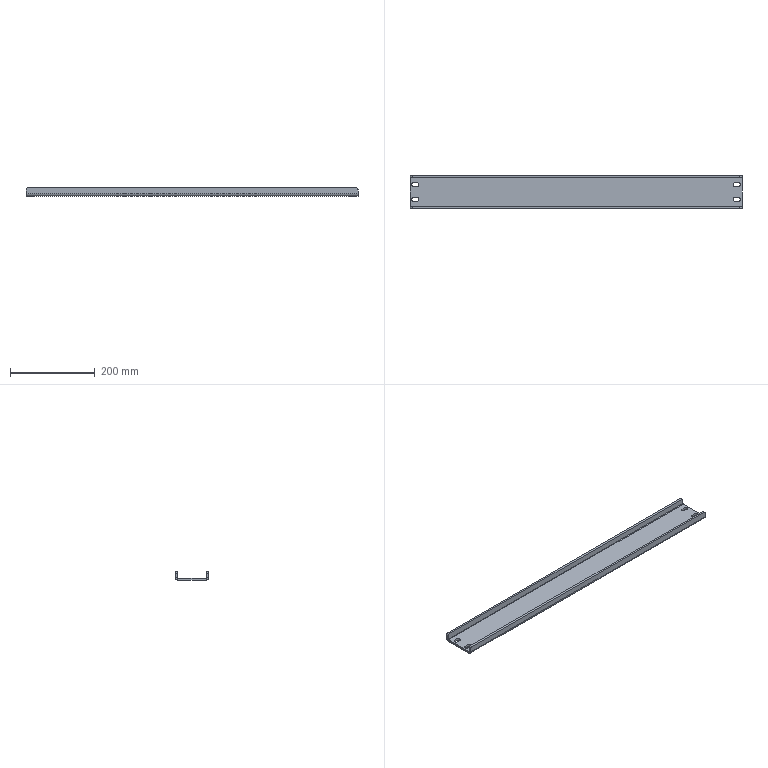Part | SolidWorks | features EdgeFlange 1, Fillet 1, FlatPattern 1, ICE 1, SMBaseFlange 1, SheetMetal 1 | 1 solid | 46 faces | box 785 x 80 x 20 mm | volume 417138 mm3 | plane 26 | cylinder 20 | commonest cylinder face diameters 9 x12 10 x4 2 x2 12 x2
STEP:
#1=CARTESIAN_POINT('',(781.,-22.5,-5.));
#2=VERTEX_POINT('',#1);
#3=CARTESIAN_POINT('',(776.5,-18.,-5.));
#4=VERTEX_POINT('',#3);
#5=CARTESIAN_POINT('',(776.5,-22.5,-5.));
#6=DIRECTION('',(0.,0.,1.));
#7=DIRECTION('',(1.,0.,0.));
#8=AXIS2_PLACEMENT_3D('',#5,#6,#7);
#9=CIRCLE('',#8,4.5);
#10=EDGE_CURVE('',#2,#4,#9,.T.);
#11=ORIENTED_EDGE('',*,*,#10,.F.);
#12=CARTESIAN_POINT('',(781.,-22.5,0.));
#13=VERTEX_POINT('',#12);
#14=CARTESIAN_POINT('',(781.,-22.5,-10.));
#15=DIRECTION('',(0.,0.,1.));
#16=VECTOR('',#15,1000.);
#17=LINE('',#14,#16);
#18=EDGE_CURVE('',#2,#13,#17,.T.);
#19=ORIENTED_EDGE('',*,*,#18,.T.);
#20=CARTESIAN_POINT('',(776.5,-18.,0.));
#21=VERTEX_POINT('',#20);
#22=CARTESIAN_POINT('',(776.5,-22.5,0.));
#23=DIRECTION('',(0.,0.,1.));
#24=DIRECTION('',(-1.,0.,0.));
#25=AXIS2_PLACEMENT_3D('',#22,#23,#24);
#26=CIRCLE('',#25,4.5);
#27=EDGE_CURVE('',#13,#21,#26,.T.);
#28=ORIENTED_EDGE('',*,*,#27,.T.);
#29=CARTESIAN_POINT('',(776.5,-18.,-10.));
#30=DIRECTION('',(0.,0.,1.));
#31=VECTOR('',#30,1000.);
#32=LINE('',#29,#31);
#33=EDGE_CURVE('',#4,#21,#32,.T.);
#34=ORIENTED_EDGE('',*,*,#33,.F.);
#35=EDGE_LOOP('',(#11,#19,#28,#34));
#36=FACE_OUTER_BOUND('',#35,.T.);
#37=CARTESIAN_POINT('',(776.5,-22.5,-10.));
#38=DIRECTION('',(0.,0.,1.));
#39=DIRECTION('',(1.,0.,0.));
#40=AXIS2_PLACEMENT_3D('',#37,#38,#39);
#41=CYLINDRICAL_SURFACE('',#40,4.5);
#42=ADVANCED_FACE('',(#36),#41,.F.);
#43=CARTESIAN_POINT('',(781.,-57.5,-5.));
#44=VERTEX_POINT('',#43);
#45=CARTESIAN_POINT('',(776.5,-53.,-5.));
#46=VERTEX_POINT('',#45);
#47=CARTESIAN_POINT('',(776.5,-57.5,-5.));
#48=DIRECTION('',(0.,0.,1.));
#49=DIRECTION('',(1.,0.,0.));
#50=AXIS2_PLACEMENT_3D('',#47,#48,#49);
#51=CIRCLE('',#50,4.5);
#52=EDGE_CURVE('',#44,#46,#51,.T.);
#53=ORIENTED_EDGE('',*,*,#52,.F.);
#54=CARTESIAN_POINT('',(781.,-57.5,0.));
#55=VERTEX_POINT('',#54);
#56=CARTESIAN_POINT('',(781.,-57.5,-10.));
#57=DIRECTION('',(0.,0.,1.));
#58=VECTOR('',#57,1000.);
#59=LINE('',#56,#58);
#60=EDGE_CURVE('',#44,#55,#59,.T.);
#61=ORIENTED_EDGE('',*,*,#60,.T.);
#62=CARTESIAN_POINT('',(776.5,-53.,0.));
#63=VERTEX_POINT('',#62);
#64=CARTESIAN_POINT('',(776.5,-57.5,0.));
#65=DIRECTION('',(0.,0.,1.));
#66=DIRECTION('',(-1.,0.,0.));
#67=AXIS2_PLACEMENT_3D('',#64,#65,#66);
#68=CIRCLE('',#67,4.5);
#69=EDGE_CURVE('',#55,#63,#68,.T.);
#70=ORIENTED_EDGE('',*,*,#69,.T.);
#71=CARTESIAN_POINT('',(776.5,-53.,-10.));
#72=DIRECTION('',(0.,0.,1.));
#73=VECTOR('',#72,1000.);
#74=LINE('',#71,#73);
#75=EDGE_CURVE('',#46,#63,#74,.T.);
#76=ORIENTED_EDGE('',*,*,#75,.F.);
#77=EDGE_LOOP('',(#53,#61,#70,#76));
#78=FACE_OUTER_BOUND('',#77,.T.);
#79=CARTESIAN_POINT('',(776.5,-57.5,-10.));
#80=DIRECTION('',(0.,0.,1.));
#81=DIRECTION('',(1.,0.,0.));
#82=AXIS2_PLACEMENT_3D('',#79,#80,#81);
#83=CYLINDRICAL_SURFACE('',#82,4.5);
#84=ADVANCED_FACE('',(#78),#83,.F.);
#85=CARTESIAN_POINT('',(21.,-57.5,-5.));
#86=VERTEX_POINT('',#85);
#87=CARTESIAN_POINT('',(16.5,-53.,-5.));
#88=VERTEX_POINT('',#87);
#89=CARTESIAN_POINT('',(16.5,-57.5,-5.));
#90=DIRECTION('',(0.,0.,1.));
#91=DIRECTION('',(1.,0.,0.));
#92=AXIS2_PLACEMENT_3D('',#89,#90,#91);
#93=CIRCLE('',#92,4.5);
#94=EDGE_CURVE('',#86,#88,#93,.T.);
#95=ORIENTED_EDGE('',*,*,#94,.F.);
#96=CARTESIAN_POINT('',(21.,-57.5,0.));
#97=VERTEX_POINT('',#96);
#98=CARTESIAN_POINT('',(21.,-57.5,-10.));
#99=DIRECTION('',(0.,0.,1.));
#100=VECTOR('',#99,1000.);
#101=LINE('',#98,#100);
#102=EDGE_CURVE('',#86,#97,#101,.T.);
#103=ORIENTED_EDGE('',*,*,#102,.T.);
#104=CARTESIAN_POINT('',(16.5,-53.,0.));
#105=VERTEX_POINT('',#104);
#106=CARTESIAN_POINT('',(16.5,-57.5,0.));
#107=DIRECTION('',(0.,0.,1.));
#108=DIRECTION('',(1.,0.,0.));
#109=AXIS2_PLACEMENT_3D('',#106,#107,#108);
#110=CIRCLE('',#109,4.5);
#111=EDGE_CURVE('',#97,#105,#110,.T.);
#112=ORIENTED_EDGE('',*,*,#111,.T.);
#113=CARTESIAN_POINT('',(16.5,-53.,-10.));
#114=DIRECTION('',(0.,0.,1.));
#115=VECTOR('',#114,1000.);
#116=LINE('',#113,#115);
#117=EDGE_CURVE('',#88,#105,#116,.T.);
#118=ORIENTED_EDGE('',*,*,#117,.F.);
#119=EDGE_LOOP('',(#95,#103,#112,#118));
#120=FACE_OUTER_BOUND('',#119,.T.);
#121=CARTESIAN_POINT('',(16.5,-57.5,-10.));
#122=DIRECTION('',(0.,0.,1.));
#123=DIRECTION('',(1.,0.,0.));
#124=AXIS2_PLACEMENT_3D('',#121,#122,#123);
#125=CYLINDRICAL_SURFACE('',#124,4.5);
#126=ADVANCED_FACE('',(#120),#125,.F.);
#127=CARTESIAN_POINT('',(21.,-22.5,-5.));
#128=VERTEX_POINT('',#127);
#129=CARTESIAN_POINT('',(16.5,-18.,-5.));
#130=VERTEX_POINT('',#129);
#131=CARTESIAN_POINT('',(16.5,-22.5,-5.));
#132=DIRECTION('',(0.,0.,1.));
#133=DIRECTION('',(1.,0.,0.));
#134=AXIS2_PLACEMENT_3D('',#131,#132,#133);
#135=CIRCLE('',#134,4.5);
#136=EDGE_CURVE('',#128,#130,#135,.T.);
#137=ORIENTED_EDGE('',*,*,#136,.F.);
#138=CARTESIAN_POINT('',(21.,-22.5,0.));
#139=VERTEX_POINT('',#138);
#140=CARTESIAN_POINT('',(21.,-22.5,-10.));
#141=DIRECTION('',(0.,0.,1.));
#142=VECTOR('',#141,1000.);
#143=LINE('',#140,#142);
#144=EDGE_CURVE('',#128,#139,#143,.T.);
#145=ORIENTED_EDGE('',*,*,#144,.T.);
#146=CARTESIAN_POINT('',(16.5,-18.,0.));
#147=VERTEX_POINT('',#146);
#148=CARTESIAN_POINT('',(16.5,-22.5,0.));
#149=DIRECTION('',(0.,0.,1.));
#150=DIRECTION('',(1.,0.,0.));
#151=AXIS2_PLACEMENT_3D('',#148,#149,#150);
#152=CIRCLE('',#151,4.5);
#153=EDGE_CURVE('',#139,#147,#152,.T.);
#154=ORIENTED_EDGE('',*,*,#153,.T.);
#155=CARTESIAN_POINT('',(16.5,-18.,-10.));
#156=DIRECTION('',(0.,0.,1.));
#157=VECTOR('',#156,1000.);
#158=LINE('',#155,#157);
#159=EDGE_CURVE('',#130,#147,#158,.T.);
#160=ORIENTED_EDGE('',*,*,#159,.F.);
#161=EDGE_LOOP('',(#137,#145,#154,#160));
#162=FACE_OUTER_BOUND('',#161,.T.);
#163=CARTESIAN_POINT('',(16.5,-22.5,-10.));
#164=DIRECTION('',(0.,0.,1.));
#165=DIRECTION('',(1.,0.,0.));
#166=AXIS2_PLACEMENT_3D('',#163,#164,#165);
#167=CYLINDRICAL_SURFACE('',#166,4.5);
#168=ADVANCED_FACE('',(#162),#167,.F.);
#169=CARTESIAN_POINT('',(768.5,-27.,-5.));
#170=VERTEX_POINT('',#169);
#171=CARTESIAN_POINT('',(776.5,-27.,-5.));
#172=VERTEX_POINT('',#171);
#173=CARTESIAN_POINT('',(0.,-27.,-5.));
#174=DIRECTION('',(1.,0.,0.));
#175=VECTOR('',#174,1000.);
#176=LINE('',#173,#175);
#177=EDGE_CURVE('',#170,#172,#176,.T.);
#178=ORIENTED_EDGE('',*,*,#177,.T.);
#179=CARTESIAN_POINT('',(776.5,-22.5,-5.));
#180=DIRECTION('',(0.,0.,1.));
#181=DIRECTION('',(1.,0.,0.));
#182=AXIS2_PLACEMENT_3D('',#179,#180,#181);
#183=CIRCLE('',#182,4.5);
#184=EDGE_CURVE('',#172,#2,#183,.T.);
#185=ORIENTED_EDGE('',*,*,#184,.T.);
#186=ORIENTED_EDGE('',*,*,#10,.T.);
#187=CARTESIAN_POINT('',(768.5,-18.,-5.));
#188=VERTEX_POINT('',#187);
#189=CARTESIAN_POINT('',(0.,-18.,-5.));
#190=DIRECTION('',(-1.,0.,0.));
#191=VECTOR('',#190,1000.);
#192=LINE('',#189,#191);
#193=EDGE_CURVE('',#4,#188,#192,.T.);
#194=ORIENTED_EDGE('',*,*,#193,.T.);
#195=CARTESIAN_POINT('',(768.5,-22.5,-5.));
#196=DIRECTION('',(0.,0.,1.));
#197=DIRECTION('',(1.,0.,0.));
#198=AXIS2_PLACEMENT_3D('',#195,#196,#197);
#199=CIRCLE('',#198,4.5);
#200=EDGE_CURVE('',#188,#170,#199,.T.);
#201=ORIENTED_EDGE('',*,*,#200,.T.);
#202=EDGE_LOOP('',(#178,#185,#186,#194,#201));
#203=FACE_BOUND('',#202,.T.);
#204=CARTESIAN_POINT('',(768.5,-62.,-5.));
#205=VERTEX_POINT('',#204);
#206=CARTESIAN_POINT('',(776.5,-62.,-5.));
#207=VERTEX_POINT('',#206);
#208=CARTESIAN_POINT('',(0.,-62.,-5.));
#209=DIRECTION('',(1.,0.,0.));
#210=VECTOR('',#209,1000.);
#211=LINE('',#208,#210);
#212=EDGE_CURVE('',#205,#207,#211,.T.);
#213=ORIENTED_EDGE('',*,*,#212,.T.);
#214=CARTESIAN_POINT('',(776.5,-57.5,-5.));
#215=DIRECTION('',(0.,0.,1.));
#216=DIRECTION('',(1.,0.,0.));
#217=AXIS2_PLACEMENT_3D('',#214,#215,#216);
#218=CIRCLE('',#217,4.5);
#219=EDGE_CURVE('',#207,#44,#218,.T.);
#220=ORIENTED_EDGE('',*,*,#219,.T.);
#221=ORIENTED_EDGE('',*,*,#52,.T.);
#222=CARTESIAN_POINT('',(768.5,-53.,-5.));
#223=VERTEX_POINT('',#222);
#224=CARTESIAN_POINT('',(0.,-53.,-5.));
#225=DIRECTION('',(-1.,0.,0.));
#226=VECTOR('',#225,1000.);
#227=LINE('',#224,#226);
#228=EDGE_CURVE('',#46,#223,#227,.T.);
#229=ORIENTED_EDGE('',*,*,#228,.T.);
#230=CARTESIAN_POINT('',(768.5,-57.5,-5.));
#231=DIRECTION('',(0.,0.,1.));
#232=DIRECTION('',(1.,0.,0.));
#233=AXIS2_PLACEMENT_3D('',#230,#231,#232);
#234=CIRCLE('',#233,4.5);
#235=EDGE_CURVE('',#223,#205,#234,.T.);
#236=ORIENTED_EDGE('',*,*,#235,.T.);
#237=EDGE_LOOP('',(#213,#220,#221,#229,#236));
#238=FACE_BOUND('',#237,.T.);
#239=CARTESIAN_POINT('',(8.5,-53.,-5.));
#240=VERTEX_POINT('',#239);
#241=CARTESIAN_POINT('',(0.,-53.,-5.));
#242=DIRECTION('',(-1.,0.,0.));
#243=VECTOR('',#242,1000.);
#244=LINE('',#241,#243);
#245=EDGE_CURVE('',#88,#240,#244,.T.);
#246=ORIENTED_EDGE('',*,*,#245,.T.);
#247=CARTESIAN_POINT('',(8.5,-62.,-5.));
#248=VERTEX_POINT('',#247);
#249=CARTESIAN_POINT('',(8.5,-57.5,-5.));
#250=DIRECTION('',(0.,0.,1.));
#251=DIRECTION('',(1.,0.,0.));
#252=AXIS2_PLACEMENT_3D('',#249,#250,#251);
#253=CIRCLE('',#252,4.5);
#254=EDGE_CURVE('',#240,#248,#253,.T.);
#255=ORIENTED_EDGE('',*,*,#254,.T.);
#256=CARTESIAN_POINT('',(16.5,-62.,-5.));
#257=VERTEX_POINT('',#256);
#258=CARTESIAN_POINT('',(0.,-62.,-5.));
#259=DIRECTION('',(1.,0.,0.));
#260=VECTOR('',#259,1000.);
#261=LINE('',#258,#260);
#262=EDGE_CURVE('',#248,#257,#261,.T.);
#263=ORIENTED_EDGE('',*,*,#262,.T.);
#264=CARTESIAN_POINT('',(16.5,-57.5,-5.));
#265=DIRECTION('',(0.,0.,1.));
#266=DIRECTION('',(1.,0.,0.));
#267=AXIS2_PLACEMENT_3D('',#264,#265,#266);
#268=CIRCLE('',#267,4.5);
#269=EDGE_CURVE('',#257,#86,#268,.T.);
#270=ORIENTED_EDGE('',*,*,#269,.T.);
#271=ORIENTED_EDGE('',*,*,#94,.T.);
#272=EDGE_LOOP('',(#246,#255,#263,#270,#271));
#273=FACE_BOUND('',#272,.T.);
#274=CARTESIAN_POINT('',(8.5,-18.,-5.));
#275=VERTEX_POINT('',#274);
#276=CARTESIAN_POINT('',(0.,-18.,-5.));
#277=DIRECTION('',(-1.,0.,0.));
#278=VECTOR('',#277,1000.);
#279=LINE('',#276,#278);
#280=EDGE_CURVE('',#130,#275,#279,.T.);
#281=ORIENTED_EDGE('',*,*,#280,.T.);
#282=CARTESIAN_POINT('',(8.5,-27.,-5.));
#283=VERTEX_POINT('',#282);
#284=CARTESIAN_POINT('',(8.5,-22.5,-5.));
#285=DIRECTION('',(0.,0.,1.));
#286=DIRECTION('',(1.,0.,0.));
#287=AXIS2_PLACEMENT_3D('',#284,#285,#286);
#288=CIRCLE('',#287,4.5);
#289=EDGE_CURVE('',#275,#283,#288,.T.);
#290=ORIENTED_EDGE('',*,*,#289,.T.);
#291=CARTESIAN_POINT('',(16.5,-27.,-5.));
#292=VERTEX_POINT('',#291);
#293=CARTESIAN_POINT('',(0.,-27.,-5.));
#294=DIRECTION('',(1.,0.,0.));
#295=VECTOR('',#294,1000.);
#296=LINE('',#293,#295);
#297=EDGE_CURVE('',#283,#292,#296,.T.);
#298=ORIENTED_EDGE('',*,*,#297,.T.);
#299=CARTESIAN_POINT('',(16.5,-22.5,-5.));
#300=DIRECTION('',(0.,0.,1.));
#301=DIRECTION('',(1.,0.,0.));
#302=AXIS2_PLACEMENT_3D('',#299,#300,#301);
#303=CIRCLE('',#302,4.5);
#304=EDGE_CURVE('',#292,#128,#303,.T.);
#305=ORIENTED_EDGE('',*,*,#304,.T.);
#306=ORIENTED_EDGE('',*,*,#136,.T.);
#307=EDGE_LOOP('',(#281,#290,#298,#305,#306));
#308=FACE_BOUND('',#307,.T.);
#309=CARTESIAN_POINT('',(785.,-74.,-5.));
#310=VERTEX_POINT('',#309);
#311=CARTESIAN_POINT('',(0.,-74.,-5.));
#312=VERTEX_POINT('',#311);
#313=CARTESIAN_POINT('',(785.,-74.,-5.));
#314=DIRECTION('',(-1.,0.,0.));
#315=VECTOR('',#314,1000.);
#316=LINE('',#313,#315);
#317=EDGE_CURVE('',#310,#312,#316,.T.);
#318=ORIENTED_EDGE('',*,*,#317,.T.);
#319=CARTESIAN_POINT('',(0.,-6.,-5.));
#320=VERTEX_POINT('',#319);
#321=CARTESIAN_POINT('',(0.,0.,-5.));
#322=DIRECTION('',(0.,-1.,0.));
#323=VECTOR('',#322,1000.);
#324=LINE('',#321,#323);
#325=EDGE_CURVE('',#320,#312,#324,.T.);
#326=ORIENTED_EDGE('',*,*,#325,.F.);
#327=CARTESIAN_POINT('',(785.,-6.,-5.));
#328=VERTEX_POINT('',#327);
#329=CARTESIAN_POINT('',(0.,-6.,-5.));
#330=DIRECTION('',(1.,0.,0.));
#331=VECTOR('',#330,1000.);
#332=LINE('',#329,#331);
#333=EDGE_CURVE('',#320,#328,#332,.T.);
#334=ORIENTED_EDGE('',*,*,#333,.T.);
#335=CARTESIAN_POINT('',(785.,0.,-5.));
#336=DIRECTION('',(0.,1.,0.));
#337=VECTOR('',#336,1000.);
#338=LINE('',#335,#337);
#339=EDGE_CURVE('',#310,#328,#338,.T.);
#340=ORIENTED_EDGE('',*,*,#339,.F.);
#341=EDGE_LOOP('',(#318,#326,#334,#340));
#342=FACE_OUTER_BOUND('',#341,.T.);
#343=CARTESIAN_POINT('',(0.,0.,-5.));
#344=DIRECTION('',(0.,0.,1.));
#345=DIRECTION('',(1.,0.,0.));
#346=AXIS2_PLACEMENT_3D('',#343,#344,#345);
#347=PLANE('',#346);
#348=ADVANCED_FACE('',(#203,#238,#273,#308,#342),#347,.F.);
#349=CARTESIAN_POINT('',(776.5,-27.,0.));
#350=VERTEX_POINT('',#349);
#351=CARTESIAN_POINT('',(776.5,-22.5,0.));
#352=DIRECTION('',(0.,0.,1.));
#353=DIRECTION('',(-1.,0.,0.));
#354=AXIS2_PLACEMENT_3D('',#351,#352,#353);
#355=CIRCLE('',#354,4.5);
#356=EDGE_CURVE('',#350,#13,#355,.T.);
#357=ORIENTED_EDGE('',*,*,#356,.F.);
#358=CARTESIAN_POINT('',(768.5,-27.,0.));
#359=VERTEX_POINT('',#358);
#360=CARTESIAN_POINT('',(776.5,-27.,0.));
#361=DIRECTION('',(1.,0.,0.));
#362=VECTOR('',#361,1000.);
#363=LINE('',#360,#362);
#364=EDGE_CURVE('',#359,#350,#363,.T.);
#365=ORIENTED_EDGE('',*,*,#364,.F.);
#366=CARTESIAN_POINT('',(768.5,-18.,0.));
#367=VERTEX_POINT('',#366);
#368=CARTESIAN_POINT('',(768.5,-22.5,0.));
#369=DIRECTION('',(0.,0.,1.));
#370=DIRECTION('',(-1.,0.,0.));
#371=AXIS2_PLACEMENT_3D('',#368,#369,#370);
#372=CIRCLE('',#371,4.5);
#373=EDGE_CURVE('',#367,#359,#372,.T.);
#374=ORIENTED_EDGE('',*,*,#373,.F.);
#375=CARTESIAN_POINT('',(776.5,-18.,0.));
#376=DIRECTION('',(-1.,0.,0.));
#377=VECTOR('',#376,1000.);
#378=LINE('',#375,#377);
#379=EDGE_CURVE('',#21,#367,#378,.T.);
#380=ORIENTED_EDGE('',*,*,#379,.F.);
#381=ORIENTED_EDGE('',*,*,#27,.F.);
#382=EDGE_LOOP('',(#357,#365,#374,#380,#381));
#383=FACE_BOUND('',#382,.T.);
#384=CARTESIAN_POINT('',(776.5,-62.,0.));
#385=VERTEX_POINT('',#384);
#386=CARTESIAN_POINT('',(776.5,-57.5,0.));
#387=DIRECTION('',(0.,0.,1.));
#388=DIRECTION('',(-1.,0.,0.));
#389=AXIS2_PLACEMENT_3D('',#386,#387,#388);
#390=CIRCLE('',#389,4.5);
#391=EDGE_CURVE('',#385,#55,#390,.T.);
#392=ORIENTED_EDGE('',*,*,#391,.F.);
#393=CARTESIAN_POINT('',(768.5,-62.,0.));
#394=VERTEX_POINT('',#393);
#395=CARTESIAN_POINT('',(776.5,-62.,0.));
#396=DIRECTION('',(1.,0.,0.));
#397=VECTOR('',#396,1000.);
#398=LINE('',#395,#397);
#399=EDGE_CURVE('',#394,#385,#398,.T.);
#400=ORIENTED_EDGE('',*,*,#399,.F.);
#401=CARTESIAN_POINT('',(768.5,-53.,0.));
#402=VERTEX_POINT('',#401);
#403=CARTESIAN_POINT('',(768.5,-57.5,0.));
#404=DIRECTION('',(0.,0.,1.));
#405=DIRECTION('',(-1.,0.,0.));
#406=AXIS2_PLACEMENT_3D('',#403,#404,#405);
#407=CIRCLE('',#406,4.5);
#408=EDGE_CURVE('',#402,#394,#407,.T.);
#409=ORIENTED_EDGE('',*,*,#408,.F.);
#410=CARTESIAN_POINT('',(776.5,-53.,0.));
#411=DIRECTION('',(-1.,0.,0.));
#412=VECTOR('',#411,1000.);
#413=LINE('',#410,#412);
#414=EDGE_CURVE('',#63,#402,#413,.T.);
#415=ORIENTED_EDGE('',*,*,#414,.F.);
#416=ORIENTED_EDGE('',*,*,#69,.F.);
#417=EDGE_LOOP('',(#392,#400,#409,#415,#416));
#418=FACE_BOUND('',#417,.T.);
#419=CARTESIAN_POINT('',(8.5,-53.,0.));
#420=VERTEX_POINT('',#419);
#421=CARTESIAN_POINT('',(8.5,-62.,0.));
#422=VERTEX_POINT('',#421);
#423=CARTESIAN_POINT('',(8.5,-57.5,0.));
#424=DIRECTION('',(0.,0.,1.));
#425=DIRECTION('',(1.,0.,0.));
#426=AXIS2_PLACEMENT_3D('',#423,#424,#425);
#427=CIRCLE('',#426,4.5);
#428=EDGE_CURVE('',#420,#422,#427,.T.);
#429=ORIENTED_EDGE('',*,*,#428,.F.);
#430=CARTESIAN_POINT('',(8.5,-53.,0.));
#431=DIRECTION('',(-1.,0.,0.));
#432=VECTOR('',#431,1000.);
#433=LINE('',#430,#432);
#434=EDGE_CURVE('',#105,#420,#433,.T.);
#435=ORIENTED_EDGE('',*,*,#434,.F.);
#436=ORIENTED_EDGE('',*,*,#111,.F.);
#437=CARTESIAN_POINT('',(16.5,-62.,0.));
#438=VERTEX_POINT('',#437);
#439=CARTESIAN_POINT('',(16.5,-57.5,0.));
#440=DIRECTION('',(0.,0.,1.));
#441=DIRECTION('',(1.,0.,0.));
#442=AXIS2_PLACEMENT_3D('',#439,#440,#441);
#443=CIRCLE('',#442,4.5);
#444=EDGE_CURVE('',#438,#97,#443,.T.);
#445=ORIENTED_EDGE('',*,*,#444,.F.);
#446=CARTESIAN_POINT('',(8.5,-62.,0.));
#447=DIRECTION('',(1.,0.,0.));
#448=VECTOR('',#447,1000.);
#449=LINE('',#446,#448);
#450=EDGE_CURVE('',#422,#438,#449,.T.);
#451=ORIENTED_EDGE('',*,*,#450,.F.);
#452=EDGE_LOOP('',(#429,#435,#436,#445,#451));
#453=FACE_BOUND('',#452,.T.);
#454=CARTESIAN_POINT('',(8.5,-18.,0.));
#455=VERTEX_POINT('',#454);
#456=CARTESIAN_POINT('',(8.5,-27.,0.));
#457=VERTEX_POINT('',#456);
#458=CARTESIAN_POINT('',(8.5,-22.5,0.));
#459=DIRECTION('',(0.,0.,1.));
#460=DIRECTION('',(1.,0.,0.));
#461=AXIS2_PLACEMENT_3D('',#458,#459,#460);
#462=CIRCLE('',#461,4.5);
#463=EDGE_CURVE('',#455,#457,#462,.T.);
#464=ORIENTED_EDGE('',*,*,#463,.F.);
#465=CARTESIAN_POINT('',(8.5,-18.,0.));
#466=DIRECTION('',(-1.,0.,0.));
#467=VECTOR('',#466,1000.);
#468=LINE('',#465,#467);
#469=EDGE_CURVE('',#147,#455,#468,.T.);
#470=ORIENTED_EDGE('',*,*,#469,.F.);
#471=ORIENTED_EDGE('',*,*,#153,.F.);
#472=CARTESIAN_POINT('',(16.5,-27.,0.));
#473=VERTEX_POINT('',#472);
#474=CARTESIAN_POINT('',(16.5,-22.5,0.));
#475=DIRECTION('',(0.,0.,1.));
#476=DIRECTION('',(1.,0.,0.));
#477=AXIS2_PLACEMENT_3D('',#474,#475,#476);
#478=CIRCLE('',#477,4.5);
#479=EDGE_CURVE('',#473,#139,#478,.T.);
#480=ORIENTED_EDGE('',*,*,#479,.F.);
#481=CARTESIAN_POINT('',(8.5,-27.,0.));
#482=DIRECTION('',(1.,0.,0.));
#483=VECTOR('',#482,1000.);
#484=LINE('',#481,#483);
#485=EDGE_CURVE('',#457,#473,#484,.T.);
#486=ORIENTED_EDGE('',*,*,#485,.F.);
#487=EDGE_LOOP('',(#464,#470,#471,#480,#486));
#488=FACE_BOUND('',#487,.T.);
#489=CARTESIAN_POINT('',(0.,-6.,0.));
#490=VERTEX_POINT('',#489);
#491=CARTESIAN_POINT('',(0.,-74.,0.));
#492=VERTEX_POINT('',#491);
#493=CARTESIAN_POINT('',(0.,0.,0.));
#494=DIRECTION('',(0.,-1.,0.));
#495=VECTOR('',#494,1000.);
#496=LINE('',#493,#495);
#497=EDGE_CURVE('',#490,#492,#496,.T.);
#498=ORIENTED_EDGE('',*,*,#497,.T.);
#499=CARTESIAN_POINT('',(785.,-74.,0.));
#500=VERTEX_POINT('',#499);
#501=CARTESIAN_POINT('',(785.,-74.,0.));
#502=DIRECTION('',(-1.,0.,0.));
#503=VECTOR('',#502,1000.);
#504=LINE('',#501,#503);
#505=EDGE_CURVE('',#500,#492,#504,.T.);
#506=ORIENTED_EDGE('',*,*,#505,.F.);
#507=CARTESIAN_POINT('',(785.,-6.,0.));
#508=VERTEX_POINT('',#507);
#509=CARTESIAN_POINT('',(785.,0.,0.));
#510=DIRECTION('',(0.,1.,0.));
#511=VECTOR('',#510,1000.);
#512=LINE('',#509,#511);
#513=EDGE_CURVE('',#500,#508,#512,.T.);
#514=ORIENTED_EDGE('',*,*,#513,.T.);
#515=CARTESIAN_POINT('',(0.,-6.,0.));
#516=DIRECTION('',(1.,0.,0.));
#517=VECTOR('',#516,1000.);
#518=LINE('',#515,#517);
#519=EDGE_CURVE('',#490,#508,#518,.T.);
#520=ORIENTED_EDGE('',*,*,#519,.F.);
#521=EDGE_LOOP('',(#498,#506,#514,#520));
#522=FACE_OUTER_BOUND('',#521,.T.);
#523=CARTESIAN_POINT('',(0.,0.,0.));
#524=DIRECTION('',(0.,0.,1.));
#525=DIRECTION('',(1.,0.,0.));
#526=AXIS2_PLACEMENT_3D('',#523,#524,#525);
#527=PLANE('',#526);
#528=ADVANCED_FACE('',(#383,#418,#453,#488,#522),#527,.T.);
#529=ORIENTED_EDGE('',*,*,#513,.F.);
#530=CARTESIAN_POINT('',(785.,-74.,0.));
#531=DIRECTION('',(0.,0.,-1.));
#532=VECTOR('',#531,1000.);
#533=LINE('',#530,#532);
#534=EDGE_CURVE('',#500,#310,#533,.T.);
#535=ORIENTED_EDGE('',*,*,#534,.T.);
#536=ORIENTED_EDGE('',*,*,#339,.T.);
#537=CARTESIAN_POINT('',(785.,-6.,0.));
#538=DIRECTION('',(0.,0.,-1.));
#539=VECTOR('',#538,1000.);
#540=LINE('',#537,#539);
#541=EDGE_CURVE('',#508,#328,#540,.T.);
#542=ORIENTED_EDGE('',*,*,#541,.F.);
#543=EDGE_LOOP('',(#529,#535,#536,#542));
#544=FACE_OUTER_BOUND('',#543,.T.);
#545=CARTESIAN_POINT('',(785.,0.,-5.));
#546=DIRECTION('',(1.,0.,0.));
#547=DIRECTION('',(0.,0.,-1.));
#548=AXIS2_PLACEMENT_3D('',#545,#546,#547);
#549=PLANE('',#548);
#550=ADVANCED_FACE('',(#544),#549,.T.);
#551=CARTESIAN_POINT('',(0.,-74.,0.));
#552=DIRECTION('',(0.,0.,-1.));
#553=VECTOR('',#552,1000.);
#554=LINE('',#551,#553);
#555=EDGE_CURVE('',#492,#312,#554,.T.);
#556=ORIENTED_EDGE('',*,*,#555,.F.);
#557=ORIENTED_EDGE('',*,*,#497,.F.);
#558=CARTESIAN_POINT('',(0.,-6.,0.));
#559=DIRECTION('',(0.,0.,-1.));
#560=VECTOR('',#559,1000.);
#561=LINE('',#558,#560);
#562=EDGE_CURVE('',#490,#320,#561,.T.);
#563=ORIENTED_EDGE('',*,*,#562,.T.);
#564=ORIENTED_EDGE('',*,*,#325,.T.);
#565=EDGE_LOOP('',(#556,#557,#563,#564));
#566=FACE_OUTER_BOUND('',#565,.T.);
#567=CARTESIAN_POINT('',(0.,0.,-5.));
#568=DIRECTION('',(-1.,0.,0.));
#569=DIRECTION('',(0.,-1.,0.));
#570=AXIS2_PLACEMENT_3D('',#567,#568,#569);
#571=PLANE('',#570);
#572=ADVANCED_FACE('',(#566),#571,.T.);
#573=CARTESIAN_POINT('',(785.,-5.,1.));
#574=VERTEX_POINT('',#573);
#575=CARTESIAN_POINT('',(785.,0.,1.));
#576=VERTEX_POINT('',#575);
#577=CARTESIAN_POINT('',(785.,0.,1.));
#578=DIRECTION('',(0.,1.,0.));
#579=VECTOR('',#578,1000.);
#580=LINE('',#577,#579);
#581=EDGE_CURVE('',#574,#576,#580,.T.);
#582=ORIENTED_EDGE('',*,*,#581,.F.);
#583=CARTESIAN_POINT('',(785.,-6.,1.));
#584=DIRECTION('',(1.,0.,0.));
#585=DIRECTION('',(0.,0.,1.));
#586=AXIS2_PLACEMENT_3D('',#583,#584,#585);
#587=CIRCLE('',#586,1.);
#588=EDGE_CURVE('',#508,#574,#587,.T.);
#589=ORIENTED_EDGE('',*,*,#588,.F.);
#590=ORIENTED_EDGE('',*,*,#541,.T.);
#591=CARTESIAN_POINT('',(785.,-6.,1.));
#592=DIRECTION('',(1.,0.,0.));
#593=DIRECTION('',(0.,0.,1.));
#594=AXIS2_PLACEMENT_3D('',#591,#592,#593);
#595=CIRCLE('',#594,6.);
#596=EDGE_CURVE('',#328,#576,#595,.T.);
#597=ORIENTED_EDGE('',*,*,#596,.T.);
#598=EDGE_LOOP('',(#582,#589,#590,#597));
#599=FACE_OUTER_BOUND('',#598,.T.);
#600=CARTESIAN_POINT('',(785.,-6.,1.));
#601=DIRECTION('',(1.,0.,0.));
#602=DIRECTION('',(0.,0.,-1.));
#603=AXIS2_PLACEMENT_3D('',#600,#601,#602);
#604=PLANE('',#603);
#605=ADVANCED_FACE('',(#599),#604,.T.);
#606=CARTESIAN_POINT('',(0.,-5.,1.));
#607=VERTEX_POINT('',#606);
#608=CARTESIAN_POINT('',(0.,-6.,1.));
#609=DIRECTION('',(-1.,0.,0.));
#610=DIRECTION('',(0.,0.,1.));
#611=AXIS2_PLACEMENT_3D('',#608,#609,#610);
#612=CIRCLE('',#611,1.);
#613=EDGE_CURVE('',#607,#490,#612,.T.);
#614=ORIENTED_EDGE('',*,*,#613,.F.);
#615=CARTESIAN_POINT('',(0.,0.,1.));
#616=VERTEX_POINT('',#615);
#617=CARTESIAN_POINT('',(0.,-5.,1.));
#618=DIRECTION('',(0.,1.,0.));
#619=VECTOR('',#618,1000.);
#620=LINE('',#617,#619);
#621=EDGE_CURVE('',#607,#616,#620,.T.);
#622=ORIENTED_EDGE('',*,*,#621,.T.);
#623=CARTESIAN_POINT('',(0.,-6.,1.));
#624=DIRECTION('',(-1.,0.,0.));
#625=DIRECTION('',(0.,0.,1.));
#626=AXIS2_PLACEMENT_3D('',#623,#624,#625);
#627=CIRCLE('',#626,6.);
#628=EDGE_CURVE('',#616,#320,#627,.T.);
#629=ORIENTED_EDGE('',*,*,#628,.T.);
#630=ORIENTED_EDGE('',*,*,#562,.F.);
#631=EDGE_LOOP('',(#614,#622,#629,#630));
#632=FACE_OUTER_BOUND('',#631,.T.);
#633=CARTESIAN_POINT('',(0.,-6.,1.));
#634=DIRECTION('',(1.,0.,0.));
#635=DIRECTION('',(0.,0.,-1.));
#636=AXIS2_PLACEMENT_3D('',#633,#634,#635);
#637=PLANE('',#636);
#638=ADVANCED_FACE('',(#632),#637,.F.);
#639=ORIENTED_EDGE('',*,*,#333,.F.);
#640=ORIENTED_EDGE('',*,*,#628,.F.);
#641=CARTESIAN_POINT('',(785.,0.,1.));
#642=DIRECTION('',(1.,0.,0.));
#643=VECTOR('',#642,1000.);
#644=LINE('',#641,#643);
#645=EDGE_CURVE('',#616,#576,#644,.T.);
#646=ORIENTED_EDGE('',*,*,#645,.T.);
#647=ORIENTED_EDGE('',*,*,#596,.F.);
#648=EDGE_LOOP('',(#639,#640,#646,#647));
#649=FACE_OUTER_BOUND('',#648,.T.);
#650=CARTESIAN_POINT('',(0.,-6.,1.));
#651=DIRECTION('',(-1.,0.,0.));
#652=DIRECTION('',(0.,1.,0.));
#653=AXIS2_PLACEMENT_3D('',#650,#651,#652);
#654=CYLINDRICAL_SURFACE('',#653,6.);
#655=ADVANCED_FACE('',(#649),#654,.T.);
#656=ORIENTED_EDGE('',*,*,#519,.T.);
#657=ORIENTED_EDGE('',*,*,#588,.T.);
#658=CARTESIAN_POINT('',(785.,-5.,1.));
#659=DIRECTION('',(-1.,0.,0.));
#660=VECTOR('',#659,1000.);
#661=LINE('',#658,#660);
#662=EDGE_CURVE('',#574,#607,#661,.T.);
#663=ORIENTED_EDGE('',*,*,#662,.T.);
#664=ORIENTED_EDGE('',*,*,#613,.T.);
#665=EDGE_LOOP('',(#656,#657,#663,#664));
#666=FACE_OUTER_BOUND('',#665,.T.);
#667=CARTESIAN_POINT('',(0.,-6.,1.));
#668=DIRECTION('',(-1.,0.,0.));
#669=DIRECTION('',(0.,1.,0.));
#670=AXIS2_PLACEMENT_3D('',#667,#668,#669);
#671=CYLINDRICAL_SURFACE('',#670,1.);
#672=ADVANCED_FACE('',(#666),#671,.F.);
#673=CARTESIAN_POINT('',(785.,0.,10.));
#674=VERTEX_POINT('',#673);
#675=CARTESIAN_POINT('',(785.,0.,0.));
#676=DIRECTION('',(0.,0.,-1.));
#677=VECTOR('',#676,1000.);
#678=LINE('',#675,#677);
#679=EDGE_CURVE('',#674,#576,#678,.T.);
#680=ORIENTED_EDGE('',*,*,#679,.F.);
#681=CARTESIAN_POINT('',(785.,-5.,10.));
#682=VERTEX_POINT('',#681);
#683=CARTESIAN_POINT('',(785.,0.,10.));
#684=DIRECTION('',(0.,-1.,0.));
#685=VECTOR('',#684,1000.);
#686=LINE('',#683,#685);
#687=EDGE_CURVE('',#674,#682,#686,.T.);
#688=ORIENTED_EDGE('',*,*,#687,.T.);
#689=CARTESIAN_POINT('',(785.,-5.,0.));
#690=DIRECTION('',(0.,0.,-1.));
#691=VECTOR('',#690,1000.);
#692=LINE('',#689,#691);
#693=EDGE_CURVE('',#682,#574,#692,.T.);
#694=ORIENTED_EDGE('',*,*,#693,.T.);
#695=ORIENTED_EDGE('',*,*,#581,.T.);
#696=EDGE_LOOP('',(#680,#688,#694,#695));
#697=FACE_OUTER_BOUND('',#696,.T.);
#698=CARTESIAN_POINT('',(785.,0.,0.));
#699=DIRECTION('',(-1.,0.,0.));
#700=DIRECTION('',(0.,0.,1.));
#701=AXIS2_PLACEMENT_3D('',#698,#699,#700);
#702=PLANE('',#701);
#703=ADVANCED_FACE('',(#697),#702,.F.);
#704=CARTESIAN_POINT('',(0.,-5.,10.));
#705=VERTEX_POINT('',#704);
#706=CARTESIAN_POINT('',(0.,-5.,15.));
#707=DIRECTION('',(0.,0.,1.));
#708=VECTOR('',#707,1000.);
#709=LINE('',#706,#708);
#710=EDGE_CURVE('',#607,#705,#709,.T.);
#711=ORIENTED_EDGE('',*,*,#710,.T.);
#712=CARTESIAN_POINT('',(0.,0.,10.));
#713=VERTEX_POINT('',#712);
#714=CARTESIAN_POINT('',(0.,0.,10.));
#715=DIRECTION('',(0.,1.,0.));
#716=VECTOR('',#715,1000.);
#717=LINE('',#714,#716);
#718=EDGE_CURVE('',#705,#713,#717,.T.);
#719=ORIENTED_EDGE('',*,*,#718,.T.);
#720=CARTESIAN_POINT('',(0.,0.,0.));
#721=DIRECTION('',(0.,0.,1.));
#722=VECTOR('',#721,1000.);
#723=LINE('',#720,#722);
#724=EDGE_CURVE('',#616,#713,#723,.T.);
#725=ORIENTED_EDGE('',*,*,#724,.F.);
#726=ORIENTED_EDGE('',*,*,#621,.F.);
#727=EDGE_LOOP('',(#711,#719,#725,#726));
#728=FACE_OUTER_BOUND('',#727,.T.);
#729=CARTESIAN_POINT('',(0.,0.,15.));
#730=DIRECTION('',(1.,0.,0.));
#731=DIRECTION('',(0.,0.,-1.));
#732=AXIS2_PLACEMENT_3D('',#729,#730,#731);
#733=PLANE('',#732);
#734=ADVANCED_FACE('',(#728),#733,.F.);
#735=CARTESIAN_POINT('',(5.,0.,15.));
#736=VERTEX_POINT('',#735);
#737=CARTESIAN_POINT('',(780.,0.,15.));
#738=VERTEX_POINT('',#737);
#739=CARTESIAN_POINT('',(0.,0.,15.));
#740=DIRECTION('',(1.,0.,0.));
#741=VECTOR('',#740,1000.);
#742=LINE('',#739,#741);
#743=EDGE_CURVE('',#736,#738,#742,.T.);
#744=ORIENTED_EDGE('',*,*,#743,.T.);
#745=CARTESIAN_POINT('',(780.,0.,10.));
#746=DIRECTION('',(0.,1.,0.));
#747=DIRECTION('',(0.,0.,-1.));
#748=AXIS2_PLACEMENT_3D('',#745,#746,#747);
#749=CIRCLE('',#748,5.);
#750=EDGE_CURVE('',#738,#674,#749,.T.);
#751=ORIENTED_EDGE('',*,*,#750,.T.);
#752=ORIENTED_EDGE('',*,*,#679,.T.);
#753=ORIENTED_EDGE('',*,*,#645,.F.);
#754=ORIENTED_EDGE('',*,*,#724,.T.);
#755=CARTESIAN_POINT('',(5.,0.,10.));
#756=DIRECTION('',(0.,1.,0.));
#757=DIRECTION('',(0.,0.,-1.));
#758=AXIS2_PLACEMENT_3D('',#755,#756,#757);
#759=CIRCLE('',#758,5.);
#760=EDGE_CURVE('',#713,#736,#759,.T.);
#761=ORIENTED_EDGE('',*,*,#760,.T.);
#762=EDGE_LOOP('',(#744,#751,#752,#753,#754,#761));
#763=FACE_OUTER_BOUND('',#762,.T.);
#764=CARTESIAN_POINT('',(0.,0.,0.));
#765=DIRECTION('',(0.,-1.,0.));
#766=DIRECTION('',(0.,0.,-1.));
#767=AXIS2_PLACEMENT_3D('',#764,#765,#766);
#768=PLANE('',#767);
#769=ADVANCED_FACE('',(#763),#768,.F.);
#770=ORIENTED_EDGE('',*,*,#693,.F.);
#771=CARTESIAN_POINT('',(780.,-5.,15.));
#772=VERTEX_POINT('',#771);
#773=CARTESIAN_POINT('',(780.,-5.,10.));
#774=DIRECTION('',(0.,-1.,0.));
#775=DIRECTION('',(0.,0.,-1.));
#776=AXIS2_PLACEMENT_3D('',#773,#774,#775);
#777=CIRCLE('',#776,5.);
#778=EDGE_CURVE('',#682,#772,#777,.T.);
#779=ORIENTED_EDGE('',*,*,#778,.T.);
#780=CARTESIAN_POINT('',(5.,-5.,15.));
#781=VERTEX_POINT('',#780);
#782=CARTESIAN_POINT('',(785.,-5.,15.));
#783=DIRECTION('',(1.,0.,0.));
#784=VECTOR('',#783,1000.);
#785=LINE('',#782,#784);
#786=EDGE_CURVE('',#781,#772,#785,.T.);
#787=ORIENTED_EDGE('',*,*,#786,.F.);
#788=CARTESIAN_POINT('',(5.,-5.,10.));
#789=DIRECTION('',(0.,-1.,0.));
#790=DIRECTION('',(0.,0.,-1.));
#791=AXIS2_PLACEMENT_3D('',#788,#789,#790);
#792=CIRCLE('',#791,5.);
#793=EDGE_CURVE('',#781,#705,#792,.T.);
#794=ORIENTED_EDGE('',*,*,#793,.T.);
#795=ORIENTED_EDGE('',*,*,#710,.F.);
#796=ORIENTED_EDGE('',*,*,#662,.F.);
#797=EDGE_LOOP('',(#770,#779,#787,#794,#795,#796));
#798=FACE_OUTER_BOUND('',#797,.T.);
#799=CARTESIAN_POINT('',(0.,-5.,0.));
#800=DIRECTION('',(0.,-1.,0.));
#801=DIRECTION('',(0.,0.,-1.));
#802=AXIS2_PLACEMENT_3D('',#799,#800,#801);
#803=PLANE('',#802);
#804=ADVANCED_FACE('',(#798),#803,.T.);
#805=ORIENTED_EDGE('',*,*,#786,.T.);
#806=CARTESIAN_POINT('',(780.,0.,15.));
#807=DIRECTION('',(0.,1.,0.));
#808=VECTOR('',#807,1000.);
#809=LINE('',#806,#808);
#810=EDGE_CURVE('',#772,#738,#809,.T.);
#811=ORIENTED_EDGE('',*,*,#810,.T.);
#812=ORIENTED_EDGE('',*,*,#743,.F.);
#813=CARTESIAN_POINT('',(5.,0.,15.));
#814=DIRECTION('',(0.,-1.,0.));
#815=VECTOR('',#814,1000.);
#816=LINE('',#813,#815);
#817=EDGE_CURVE('',#736,#781,#816,.T.);
#818=ORIENTED_EDGE('',*,*,#817,.T.);
#819=EDGE_LOOP('',(#805,#811,#812,#818));
#820=FACE_OUTER_BOUND('',#819,.T.);
#821=CARTESIAN_POINT('',(785.,0.,15.));
#822=DIRECTION('',(0.,0.,-1.));
#823=DIRECTION('',(0.,1.,0.));
#824=AXIS2_PLACEMENT_3D('',#821,#822,#823);
#825=PLANE('',#824);
#826=ADVANCED_FACE('',(#820),#825,.F.);
#827=CARTESIAN_POINT('',(0.,-75.,1.));
#828=VERTEX_POINT('',#827);
#829=CARTESIAN_POINT('',(0.,-80.,1.));
#830=VERTEX_POINT('',#829);
#831=CARTESIAN_POINT('',(0.,-80.,1.));
#832=DIRECTION('',(0.,-1.,0.));
#833=VECTOR('',#832,1000.);
#834=LINE('',#831,#833);
#835=EDGE_CURVE('',#828,#830,#834,.T.);
#836=ORIENTED_EDGE('',*,*,#835,.F.);
#837=CARTESIAN_POINT('',(0.,-74.,1.));
#838=DIRECTION('',(-1.,0.,0.));
#839=DIRECTION('',(0.,0.,-1.));
#840=AXIS2_PLACEMENT_3D('',#837,#838,#839);
#841=CIRCLE('',#840,1.);
#842=EDGE_CURVE('',#492,#828,#841,.T.);
#843=ORIENTED_EDGE('',*,*,#842,.F.);
#844=ORIENTED_EDGE('',*,*,#555,.T.);
#845=CARTESIAN_POINT('',(0.,-74.,1.));
#846=DIRECTION('',(-1.,0.,0.));
#847=DIRECTION('',(0.,0.,-1.));
#848=AXIS2_PLACEMENT_3D('',#845,#846,#847);
#849=CIRCLE('',#848,6.);
#850=EDGE_CURVE('',#312,#830,#849,.T.);
#851=ORIENTED_EDGE('',*,*,#850,.T.);
#852=EDGE_LOOP('',(#836,#843,#844,#851));
#853=FACE_OUTER_BOUND('',#852,.T.);
#854=CARTESIAN_POINT('',(0.,-74.,1.));
#855=DIRECTION('',(-1.,0.,0.));
#856=DIRECTION('',(0.,0.,1.));
#857=AXIS2_PLACEMENT_3D('',#854,#855,#856);
#858=PLANE('',#857);
#859=ADVANCED_FACE('',(#853),#858,.T.);
#860=CARTESIAN_POINT('',(785.,-75.,1.));
#861=VERTEX_POINT('',#860);
#862=CARTESIAN_POINT('',(785.,-74.,1.));
#863=DIRECTION('',(1.,0.,0.));
#864=DIRECTION('',(0.,0.,-1.));
#865=AXIS2_PLACEMENT_3D('',#862,#863,#864);
#866=CIRCLE('',#865,1.);
#867=EDGE_CURVE('',#861,#500,#866,.T.);
#868=ORIENTED_EDGE('',*,*,#867,.F.);
#869=CARTESIAN_POINT('',(785.,-80.,1.));
#870=VERTEX_POINT('',#869);
#871=CARTESIAN_POINT('',(785.,-75.,1.));
#872=DIRECTION('',(0.,-1.,0.));
#873=VECTOR('',#872,1000.);
#874=LINE('',#871,#873);
#875=EDGE_CURVE('',#861,#870,#874,.T.);
#876=ORIENTED_EDGE('',*,*,#875,.T.);
#877=CARTESIAN_POINT('',(785.,-74.,1.));
#878=DIRECTION('',(1.,0.,0.));
#879=DIRECTION('',(0.,0.,-1.));
#880=AXIS2_PLACEMENT_3D('',#877,#878,#879);
#881=CIRCLE('',#880,6.);
#882=EDGE_CURVE('',#870,#310,#881,.T.);
#883=ORIENTED_EDGE('',*,*,#882,.T.);
#884=ORIENTED_EDGE('',*,*,#534,.F.);
#885=EDGE_LOOP('',(#868,#876,#883,#884));
#886=FACE_OUTER_BOUND('',#885,.T.);
#887=CARTESIAN_POINT('',(785.,-74.,1.));
#888=DIRECTION('',(-1.,0.,0.));
#889=DIRECTION('',(0.,0.,1.));
#890=AXIS2_PLACEMENT_3D('',#887,#888,#889);
#891=PLANE('',#890);
#892=ADVANCED_FACE('',(#886),#891,.F.);
#893=ORIENTED_EDGE('',*,*,#317,.F.);
#894=ORIENTED_EDGE('',*,*,#882,.F.);
#895=CARTESIAN_POINT('',(0.,-80.,1.));
#896=DIRECTION('',(-1.,0.,0.));
#897=VECTOR('',#896,1000.);
#898=LINE('',#895,#897);
#899=EDGE_CURVE('',#870,#830,#898,.T.);
#900=ORIENTED_EDGE('',*,*,#899,.T.);
#901=ORIENTED_EDGE('',*,*,#850,.F.);
#902=EDGE_LOOP('',(#893,#894,#900,#901));
#903=FACE_OUTER_BOUND('',#902,.T.);
#904=CARTESIAN_POINT('',(785.,-74.,1.));
#905=DIRECTION('',(1.,0.,0.));
#906=DIRECTION('',(0.,-1.,0.));
#907=AXIS2_PLACEMENT_3D('',#904,#905,#906);
#908=CYLINDRICAL_SURFACE('',#907,6.);
#909=ADVANCED_FACE('',(#903),#908,.T.);
#910=ORIENTED_EDGE('',*,*,#505,.T.);
#911=ORIENTED_EDGE('',*,*,#842,.T.);
#912=CARTESIAN_POINT('',(0.,-75.,1.));
#913=DIRECTION('',(1.,0.,0.));
#914=VECTOR('',#913,1000.);
#915=LINE('',#912,#914);
#916=EDGE_CURVE('',#828,#861,#915,.T.);
#917=ORIENTED_EDGE('',*,*,#916,.T.);
#918=ORIENTED_EDGE('',*,*,#867,.T.);
#919=EDGE_LOOP('',(#910,#911,#917,#918));
#920=FACE_OUTER_BOUND('',#919,.T.);
#921=CARTESIAN_POINT('',(785.,-74.,1.));
#922=DIRECTION('',(1.,0.,0.));
#923=DIRECTION('',(0.,-1.,0.));
#924=AXIS2_PLACEMENT_3D('',#921,#922,#923);
#925=CYLINDRICAL_SURFACE('',#924,1.);
#926=ADVANCED_FACE('',(#920),#925,.F.);
#927=CARTESIAN_POINT('',(0.,-80.,10.));
#928=VERTEX_POINT('',#927);
#929=CARTESIAN_POINT('',(0.,-80.,0.));
#930=DIRECTION('',(0.,0.,-1.));
#931=VECTOR('',#930,1000.);
#932=LINE('',#929,#931);
#933=EDGE_CURVE('',#928,#830,#932,.T.);
#934=ORIENTED_EDGE('',*,*,#933,.F.);
#935=CARTESIAN_POINT('',(0.,-75.,10.));
#936=VERTEX_POINT('',#935);
#937=CARTESIAN_POINT('',(0.,-80.,10.));
#938=DIRECTION('',(0.,1.,0.));
#939=VECTOR('',#938,1000.);
#940=LINE('',#937,#939);
#941=EDGE_CURVE('',#928,#936,#940,.T.);
#942=ORIENTED_EDGE('',*,*,#941,.T.);
#943=CARTESIAN_POINT('',(0.,-75.,0.));
#944=DIRECTION('',(0.,0.,-1.));
#945=VECTOR('',#944,1000.);
#946=LINE('',#943,#945);
#947=EDGE_CURVE('',#936,#828,#946,.T.);
#948=ORIENTED_EDGE('',*,*,#947,.T.);
#949=ORIENTED_EDGE('',*,*,#835,.T.);
#950=EDGE_LOOP('',(#934,#942,#948,#949));
#951=FACE_OUTER_BOUND('',#950,.T.);
#952=CARTESIAN_POINT('',(0.,-80.,0.));
#953=DIRECTION('',(1.,0.,0.));
#954=DIRECTION('',(0.,0.,-1.));
#955=AXIS2_PLACEMENT_3D('',#952,#953,#954);
#956=PLANE('',#955);
#957=ADVANCED_FACE('',(#951),#956,.F.);
#958=CARTESIAN_POINT('',(785.,-75.,10.));
#959=VERTEX_POINT('',#958);
#960=CARTESIAN_POINT('',(785.,-75.,15.));
#961=DIRECTION('',(0.,0.,1.));
#962=VECTOR('',#961,1000.);
#963=LINE('',#960,#962);
#964=EDGE_CURVE('',#861,#959,#963,.T.);
#965=ORIENTED_EDGE('',*,*,#964,.T.);
#966=CARTESIAN_POINT('',(785.,-80.,10.));
#967=VERTEX_POINT('',#966);
#968=CARTESIAN_POINT('',(785.,-80.,10.));
#969=DIRECTION('',(0.,-1.,0.));
#970=VECTOR('',#969,1000.);
#971=LINE('',#968,#970);
#972=EDGE_CURVE('',#959,#967,#971,.T.);
#973=ORIENTED_EDGE('',*,*,#972,.T.);
#974=CARTESIAN_POINT('',(785.,-80.,0.));
#975=DIRECTION('',(0.,0.,1.));
#976=VECTOR('',#975,1000.);
#977=LINE('',#974,#976);
#978=EDGE_CURVE('',#870,#967,#977,.T.);
#979=ORIENTED_EDGE('',*,*,#978,.F.);
#980=ORIENTED_EDGE('',*,*,#875,.F.);
#981=EDGE_LOOP('',(#965,#973,#979,#980));
#982=FACE_OUTER_BOUND('',#981,.T.);
#983=CARTESIAN_POINT('',(785.,-80.,15.));
#984=DIRECTION('',(-1.,0.,0.));
#985=DIRECTION('',(0.,0.,1.));
#986=AXIS2_PLACEMENT_3D('',#983,#984,#985);
#987=PLANE('',#986);
#988=ADVANCED_FACE('',(#982),#987,.F.);
#989=ORIENTED_EDGE('',*,*,#978,.T.);
#990=CARTESIAN_POINT('',(780.,-80.,15.));
#991=VERTEX_POINT('',#990);
#992=CARTESIAN_POINT('',(780.,-80.,10.));
#993=DIRECTION('',(0.,-1.,0.));
#994=DIRECTION('',(0.,0.,1.));
#995=AXIS2_PLACEMENT_3D('',#992,#993,#994);
#996=CIRCLE('',#995,5.);
#997=EDGE_CURVE('',#967,#991,#996,.T.);
#998=ORIENTED_EDGE('',*,*,#997,.T.);
#999=CARTESIAN_POINT('',(5.,-80.,15.));
#1000=VERTEX_POINT('',#999);
#1001=CARTESIAN_POINT('',(0.,-80.,15.));
#1002=DIRECTION('',(-1.,0.,0.));
#1003=VECTOR('',#1002,1000.);
#1004=LINE('',#1001,#1003);
#1005=EDGE_CURVE('',#991,#1000,#1004,.T.);
#1006=ORIENTED_EDGE('',*,*,#1005,.T.);
#1007=CARTESIAN_POINT('',(5.,-80.,10.));
#1008=DIRECTION('',(0.,-1.,0.));
#1009=DIRECTION('',(0.,0.,1.));
#1010=AXIS2_PLACEMENT_3D('',#1007,#1008,#1009);
#1011=CIRCLE('',#1010,5.);
#1012=EDGE_CURVE('',#1000,#928,#1011,.T.);
#1013=ORIENTED_EDGE('',*,*,#1012,.T.);
#1014=ORIENTED_EDGE('',*,*,#933,.T.);
#1015=ORIENTED_EDGE('',*,*,#899,.F.);
#1016=EDGE_LOOP('',(#989,#998,#1006,#1013,#1014,#1015));
#1017=FACE_OUTER_BOUND('',#1016,.T.);
#1018=CARTESIAN_POINT('',(0.,-80.,0.));
#1019=DIRECTION('',(0.,1.,0.));
#1020=DIRECTION('',(0.,0.,1.));
#1021=AXIS2_PLACEMENT_3D('',#1018,#1019,#1020);
#1022=PLANE('',#1021);
#1023=ADVANCED_FACE('',(#1017),#1022,.F.);
#1024=CARTESIAN_POINT('',(780.,-75.,15.));
#1025=VERTEX_POINT('',#1024);
#1026=CARTESIAN_POINT('',(5.,-75.,15.));
#1027=VERTEX_POINT('',#1026);
#1028=CARTESIAN_POINT('',(0.,-75.,15.));
#1029=DIRECTION('',(-1.,0.,0.));
#1030=VECTOR('',#1029,1000.);
#1031=LINE('',#1028,#1030);
#1032=EDGE_CURVE('',#1025,#1027,#1031,.T.);
#1033=ORIENTED_EDGE('',*,*,#1032,.F.);
#1034=CARTESIAN_POINT('',(780.,-75.,10.));
#1035=DIRECTION('',(0.,1.,0.));
#1036=DIRECTION('',(0.,0.,1.));
#1037=AXIS2_PLACEMENT_3D('',#1034,#1035,#1036);
#1038=CIRCLE('',#1037,5.);
#1039=EDGE_CURVE('',#1025,#959,#1038,.T.);
#1040=ORIENTED_EDGE('',*,*,#1039,.T.);
#1041=ORIENTED_EDGE('',*,*,#964,.F.);
#1042=ORIENTED_EDGE('',*,*,#916,.F.);
#1043=ORIENTED_EDGE('',*,*,#947,.F.);
#1044=CARTESIAN_POINT('',(5.,-75.,10.));
#1045=DIRECTION('',(0.,1.,0.));
#1046=DIRECTION('',(0.,0.,1.));
#1047=AXIS2_PLACEMENT_3D('',#1044,#1045,#1046);
#1048=CIRCLE('',#1047,5.);
#1049=EDGE_CURVE('',#936,#1027,#1048,.T.);
#1050=ORIENTED_EDGE('',*,*,#1049,.T.);
#1051=EDGE_LOOP('',(#1033,#1040,#1041,#1042,#1043,#1050));
#1052=FACE_OUTER_BOUND('',#1051,.T.);
#1053=CARTESIAN_POINT('',(0.,-75.,0.));
#1054=DIRECTION('',(0.,1.,0.));
#1055=DIRECTION('',(0.,0.,1.));
#1056=AXIS2_PLACEMENT_3D('',#1053,#1054,#1055);
#1057=PLANE('',#1056);
#1058=ADVANCED_FACE('',(#1052),#1057,.T.);
#1059=ORIENTED_EDGE('',*,*,#1005,.F.);
#1060=CARTESIAN_POINT('',(780.,-80.,15.));
#1061=DIRECTION('',(0.,1.,0.));
#1062=VECTOR('',#1061,1000.);
#1063=LINE('',#1060,#1062);
#1064=EDGE_CURVE('',#991,#1025,#1063,.T.);
#1065=ORIENTED_EDGE('',*,*,#1064,.T.);
#1066=ORIENTED_EDGE('',*,*,#1032,.T.);
#1067=CARTESIAN_POINT('',(5.,-80.,15.));
#1068=DIRECTION('',(0.,-1.,0.));
#1069=VECTOR('',#1068,1000.);
#1070=LINE('',#1067,#1069);
#1071=EDGE_CURVE('',#1027,#1000,#1070,.T.);
#1072=ORIENTED_EDGE('',*,*,#1071,.T.);
#1073=EDGE_LOOP('',(#1059,#1065,#1066,#1072));
#1074=FACE_OUTER_BOUND('',#1073,.T.);
#1075=CARTESIAN_POINT('',(0.,-80.,15.));
#1076=DIRECTION('',(0.,0.,-1.));
#1077=DIRECTION('',(0.,1.,0.));
#1078=AXIS2_PLACEMENT_3D('',#1075,#1076,#1077);
#1079=PLANE('',#1078);
#1080=ADVANCED_FACE('',(#1074),#1079,.F.);
#1081=CARTESIAN_POINT('',(8.5,-18.,-10.));
#1082=DIRECTION('',(0.,0.,1.));
#1083=VECTOR('',#1082,1000.);
#1084=LINE('',#1081,#1083);
#1085=EDGE_CURVE('',#275,#455,#1084,.T.);
#1086=ORIENTED_EDGE('',*,*,#1085,.T.);
#1087=ORIENTED_EDGE('',*,*,#463,.T.);
#1088=CARTESIAN_POINT('',(8.5,-27.,-10.));
#1089=DIRECTION('',(0.,0.,1.));
#1090=VECTOR('',#1089,1000.);
#1091=LINE('',#1088,#1090);
#1092=EDGE_CURVE('',#283,#457,#1091,.T.);
#1093=ORIENTED_EDGE('',*,*,#1092,.F.);
#1094=ORIENTED_EDGE('',*,*,#289,.F.);
#1095=EDGE_LOOP('',(#1086,#1087,#1093,#1094));
#1096=FACE_OUTER_BOUND('',#1095,.T.);
#1097=CARTESIAN_POINT('',(8.5,-22.5,-10.));
#1098=DIRECTION('',(0.,0.,1.));
#1099=DIRECTION('',(1.,0.,0.));
#1100=AXIS2_PLACEMENT_3D('',#1097,#1098,#1099);
#1101=CYLINDRICAL_SURFACE('',#1100,4.5);
#1102=ADVANCED_FACE('',(#1096),#1101,.F.);
#1103=ORIENTED_EDGE('',*,*,#159,.T.);
#1104=ORIENTED_EDGE('',*,*,#469,.T.);
#1105=ORIENTED_EDGE('',*,*,#1085,.F.);
#1106=ORIENTED_EDGE('',*,*,#280,.F.);
#1107=EDGE_LOOP('',(#1103,#1104,#1105,#1106));
#1108=FACE_OUTER_BOUND('',#1107,.T.);
#1109=CARTESIAN_POINT('',(8.5,-18.,-10.));
#1110=DIRECTION('',(0.,1.,0.));
#1111=DIRECTION('',(0.,0.,1.));
#1112=AXIS2_PLACEMENT_3D('',#1109,#1110,#1111);
#1113=PLANE('',#1112);
#1114=ADVANCED_FACE('',(#1108),#1113,.F.);
#1115=ORIENTED_EDGE('',*,*,#144,.F.);
#1116=ORIENTED_EDGE('',*,*,#304,.F.);
#1117=CARTESIAN_POINT('',(16.5,-27.,-10.));
#1118=DIRECTION('',(0.,0.,1.));
#1119=VECTOR('',#1118,1000.);
#1120=LINE('',#1117,#1119);
#1121=EDGE_CURVE('',#292,#473,#1120,.T.);
#1122=ORIENTED_EDGE('',*,*,#1121,.T.);
#1123=ORIENTED_EDGE('',*,*,#479,.T.);
#1124=EDGE_LOOP('',(#1115,#1116,#1122,#1123));
#1125=FACE_OUTER_BOUND('',#1124,.T.);
#1126=CARTESIAN_POINT('',(16.5,-22.5,-10.));
#1127=DIRECTION('',(0.,0.,1.));
#1128=DIRECTION('',(1.,0.,0.));
#1129=AXIS2_PLACEMENT_3D('',#1126,#1127,#1128);
#1130=CYLINDRICAL_SURFACE('',#1129,4.5);
#1131=ADVANCED_FACE('',(#1125),#1130,.F.);
#1132=ORIENTED_EDGE('',*,*,#1092,.T.);
#1133=ORIENTED_EDGE('',*,*,#485,.T.);
#1134=ORIENTED_EDGE('',*,*,#1121,.F.);
#1135=ORIENTED_EDGE('',*,*,#297,.F.);
#1136=EDGE_LOOP('',(#1132,#1133,#1134,#1135));
#1137=FACE_OUTER_BOUND('',#1136,.T.);
#1138=CARTESIAN_POINT('',(8.5,-27.,-10.));
#1139=DIRECTION('',(0.,-1.,0.));
#1140=DIRECTION('',(0.,0.,-1.));
#1141=AXIS2_PLACEMENT_3D('',#1138,#1139,#1140);
#1142=PLANE('',#1141);
#1143=ADVANCED_FACE('',(#1137),#1142,.F.);
#1144=CARTESIAN_POINT('',(8.5,-53.,-10.));
#1145=DIRECTION('',(0.,0.,1.));
#1146=VECTOR('',#1145,1000.);
#1147=LINE('',#1144,#1146);
#1148=EDGE_CURVE('',#240,#420,#1147,.T.);
#1149=ORIENTED_EDGE('',*,*,#1148,.T.);
#1150=ORIENTED_EDGE('',*,*,#428,.T.);
#1151=CARTESIAN_POINT('',(8.5,-62.,-10.));
#1152=DIRECTION('',(0.,0.,1.));
#1153=VECTOR('',#1152,1000.);
#1154=LINE('',#1151,#1153);
#1155=EDGE_CURVE('',#248,#422,#1154,.T.);
#1156=ORIENTED_EDGE('',*,*,#1155,.F.);
#1157=ORIENTED_EDGE('',*,*,#254,.F.);
#1158=EDGE_LOOP('',(#1149,#1150,#1156,#1157));
#1159=FACE_OUTER_BOUND('',#1158,.T.);
#1160=CARTESIAN_POINT('',(8.5,-57.5,-10.));
#1161=DIRECTION('',(0.,0.,1.));
#1162=DIRECTION('',(1.,0.,0.));
#1163=AXIS2_PLACEMENT_3D('',#1160,#1161,#1162);
#1164=CYLINDRICAL_SURFACE('',#1163,4.5);
#1165=ADVANCED_FACE('',(#1159),#1164,.F.);
#1166=ORIENTED_EDGE('',*,*,#117,.T.);
#1167=ORIENTED_EDGE('',*,*,#434,.T.);
#1168=ORIENTED_EDGE('',*,*,#1148,.F.);
#1169=ORIENTED_EDGE('',*,*,#245,.F.);
#1170=EDGE_LOOP('',(#1166,#1167,#1168,#1169));
#1171=FACE_OUTER_BOUND('',#1170,.T.);
#1172=CARTESIAN_POINT('',(8.5,-53.,-10.));
#1173=DIRECTION('',(0.,1.,0.));
#1174=DIRECTION('',(0.,0.,1.));
#1175=AXIS2_PLACEMENT_3D('',#1172,#1173,#1174);
#1176=PLANE('',#1175);
#1177=ADVANCED_FACE('',(#1171),#1176,.F.);
#1178=ORIENTED_EDGE('',*,*,#102,.F.);
#1179=ORIENTED_EDGE('',*,*,#269,.F.);
#1180=CARTESIAN_POINT('',(16.5,-62.,-10.));
#1181=DIRECTION('',(0.,0.,1.));
#1182=VECTOR('',#1181,1000.);
#1183=LINE('',#1180,#1182);
#1184=EDGE_CURVE('',#257,#438,#1183,.T.);
#1185=ORIENTED_EDGE('',*,*,#1184,.T.);
#1186=ORIENTED_EDGE('',*,*,#444,.T.);
#1187=EDGE_LOOP('',(#1178,#1179,#1185,#1186));
#1188=FACE_OUTER_BOUND('',#1187,.T.);
#1189=CARTESIAN_POINT('',(16.5,-57.5,-10.));
#1190=DIRECTION('',(0.,0.,1.));
#1191=DIRECTION('',(1.,0.,0.));
#1192=AXIS2_PLACEMENT_3D('',#1189,#1190,#1191);
#1193=CYLINDRICAL_SURFACE('',#1192,4.5);
#1194=ADVANCED_FACE('',(#1188),#1193,.F.);
#1195=ORIENTED_EDGE('',*,*,#1155,.T.);
#1196=ORIENTED_EDGE('',*,*,#450,.T.);
#1197=ORIENTED_EDGE('',*,*,#1184,.F.);
#1198=ORIENTED_EDGE('',*,*,#262,.F.);
#1199=EDGE_LOOP('',(#1195,#1196,#1197,#1198));
#1200=FACE_OUTER_BOUND('',#1199,.T.);
#1201=CARTESIAN_POINT('',(8.5,-62.,-10.));
#1202=DIRECTION('',(0.,-1.,0.));
#1203=DIRECTION('',(0.,0.,-1.));
#1204=AXIS2_PLACEMENT_3D('',#1201,#1202,#1203);
#1205=PLANE('',#1204);
#1206=ADVANCED_FACE('',(#1200),#1205,.F.);
#1207=ORIENTED_EDGE('',*,*,#60,.F.);
#1208=ORIENTED_EDGE('',*,*,#219,.F.);
#1209=CARTESIAN_POINT('',(776.5,-62.,-10.));
#1210=DIRECTION('',(0.,0.,1.));
#1211=VECTOR('',#1210,1000.);
#1212=LINE('',#1209,#1211);
#1213=EDGE_CURVE('',#207,#385,#1212,.T.);
#1214=ORIENTED_EDGE('',*,*,#1213,.T.);
#1215=ORIENTED_EDGE('',*,*,#391,.T.);
#1216=EDGE_LOOP('',(#1207,#1208,#1214,#1215));
#1217=FACE_OUTER_BOUND('',#1216,.T.);
#1218=CARTESIAN_POINT('',(776.5,-57.5,-10.));
#1219=DIRECTION('',(0.,0.,1.));
#1220=DIRECTION('',(1.,0.,0.));
#1221=AXIS2_PLACEMENT_3D('',#1218,#1219,#1220);
#1222=CYLINDRICAL_SURFACE('',#1221,4.5);
#1223=ADVANCED_FACE('',(#1217),#1222,.F.);
#1224=CARTESIAN_POINT('',(768.5,-62.,-10.));
#1225=DIRECTION('',(0.,0.,1.));
#1226=VECTOR('',#1225,1000.);
#1227=LINE('',#1224,#1226);
#1228=EDGE_CURVE('',#205,#394,#1227,.T.);
#1229=ORIENTED_EDGE('',*,*,#1228,.T.);
#1230=ORIENTED_EDGE('',*,*,#399,.T.);
#1231=ORIENTED_EDGE('',*,*,#1213,.F.);
#1232=ORIENTED_EDGE('',*,*,#212,.F.);
#1233=EDGE_LOOP('',(#1229,#1230,#1231,#1232));
#1234=FACE_OUTER_BOUND('',#1233,.T.);
#1235=CARTESIAN_POINT('',(776.5,-62.,-10.));
#1236=DIRECTION('',(0.,-1.,0.));
#1237=DIRECTION('',(0.,0.,-1.));
#1238=AXIS2_PLACEMENT_3D('',#1235,#1236,#1237);
#1239=PLANE('',#1238);
#1240=ADVANCED_FACE('',(#1234),#1239,.F.);
#1241=CARTESIAN_POINT('',(768.5,-53.,-10.));
#1242=DIRECTION('',(0.,0.,1.));
#1243=VECTOR('',#1242,1000.);
#1244=LINE('',#1241,#1243);
#1245=EDGE_CURVE('',#223,#402,#1244,.T.);
#1246=ORIENTED_EDGE('',*,*,#1245,.T.);
#1247=ORIENTED_EDGE('',*,*,#408,.T.);
#1248=ORIENTED_EDGE('',*,*,#1228,.F.);
#1249=ORIENTED_EDGE('',*,*,#235,.F.);
#1250=EDGE_LOOP('',(#1246,#1247,#1248,#1249));
#1251=FACE_OUTER_BOUND('',#1250,.T.);
#1252=CARTESIAN_POINT('',(768.5,-57.5,-10.));
#1253=DIRECTION('',(0.,0.,1.));
#1254=DIRECTION('',(1.,0.,0.));
#1255=AXIS2_PLACEMENT_3D('',#1252,#1253,#1254);
#1256=CYLINDRICAL_SURFACE('',#1255,4.5);
#1257=ADVANCED_FACE('',(#1251),#1256,.F.);
#1258=ORIENTED_EDGE('',*,*,#75,.T.);
#1259=ORIENTED_EDGE('',*,*,#414,.T.);
#1260=ORIENTED_EDGE('',*,*,#1245,.F.);
#1261=ORIENTED_EDGE('',*,*,#228,.F.);
#1262=EDGE_LOOP('',(#1258,#1259,#1260,#1261));
#1263=FACE_OUTER_BOUND('',#1262,.T.);
#1264=CARTESIAN_POINT('',(776.5,-53.,-10.));
#1265=DIRECTION('',(0.,1.,0.));
#1266=DIRECTION('',(0.,0.,1.));
#1267=AXIS2_PLACEMENT_3D('',#1264,#1265,#1266);
#1268=PLANE('',#1267);
#1269=ADVANCED_FACE('',(#1263),#1268,.F.);
#1270=ORIENTED_EDGE('',*,*,#18,.F.);
#1271=ORIENTED_EDGE('',*,*,#184,.F.);
#1272=CARTESIAN_POINT('',(776.5,-27.,-10.));
#1273=DIRECTION('',(0.,0.,1.));
#1274=VECTOR('',#1273,1000.);
#1275=LINE('',#1272,#1274);
#1276=EDGE_CURVE('',#172,#350,#1275,.T.);
#1277=ORIENTED_EDGE('',*,*,#1276,.T.);
#1278=ORIENTED_EDGE('',*,*,#356,.T.);
#1279=EDGE_LOOP('',(#1270,#1271,#1277,#1278));
#1280=FACE_OUTER_BOUND('',#1279,.T.);
#1281=CARTESIAN_POINT('',(776.5,-22.5,-10.));
#1282=DIRECTION('',(0.,0.,1.));
#1283=DIRECTION('',(1.,0.,0.));
#1284=AXIS2_PLACEMENT_3D('',#1281,#1282,#1283);
#1285=CYLINDRICAL_SURFACE('',#1284,4.5);
#1286=ADVANCED_FACE('',(#1280),#1285,.F.);
#1287=CARTESIAN_POINT('',(768.5,-27.,-10.));
#1288=DIRECTION('',(0.,0.,1.));
#1289=VECTOR('',#1288,1000.);
#1290=LINE('',#1287,#1289);
#1291=EDGE_CURVE('',#170,#359,#1290,.T.);
#1292=ORIENTED_EDGE('',*,*,#1291,.T.);
#1293=ORIENTED_EDGE('',*,*,#364,.T.);
#1294=ORIENTED_EDGE('',*,*,#1276,.F.);
#1295=ORIENTED_EDGE('',*,*,#177,.F.);
#1296=EDGE_LOOP('',(#1292,#1293,#1294,#1295));
#1297=FACE_OUTER_BOUND('',#1296,.T.);
#1298=CARTESIAN_POINT('',(776.5,-27.,-10.));
#1299=DIRECTION('',(0.,-1.,0.));
#1300=DIRECTION('',(0.,0.,-1.));
#1301=AXIS2_PLACEMENT_3D('',#1298,#1299,#1300);
#1302=PLANE('',#1301);
#1303=ADVANCED_FACE('',(#1297),#1302,.F.);
#1304=CARTESIAN_POINT('',(768.5,-18.,-10.));
#1305=DIRECTION('',(0.,0.,1.));
#1306=VECTOR('',#1305,1000.);
#1307=LINE('',#1304,#1306);
#1308=EDGE_CURVE('',#188,#367,#1307,.T.);
#1309=ORIENTED_EDGE('',*,*,#1308,.T.);
#1310=ORIENTED_EDGE('',*,*,#373,.T.);
#1311=ORIENTED_EDGE('',*,*,#1291,.F.);
#1312=ORIENTED_EDGE('',*,*,#200,.F.);
#1313=EDGE_LOOP('',(#1309,#1310,#1311,#1312));
#1314=FACE_OUTER_BOUND('',#1313,.T.);
#1315=CARTESIAN_POINT('',(768.5,-22.5,-10.));
#1316=DIRECTION('',(0.,0.,1.));
#1317=DIRECTION('',(1.,0.,0.));
#1318=AXIS2_PLACEMENT_3D('',#1315,#1316,#1317);
#1319=CYLINDRICAL_SURFACE('',#1318,4.5);
#1320=ADVANCED_FACE('',(#1314),#1319,.F.);
#1321=ORIENTED_EDGE('',*,*,#33,.T.);
#1322=ORIENTED_EDGE('',*,*,#379,.T.);
#1323=ORIENTED_EDGE('',*,*,#1308,.F.);
#1324=ORIENTED_EDGE('',*,*,#193,.F.);
#1325=EDGE_LOOP('',(#1321,#1322,#1323,#1324));
#1326=FACE_OUTER_BOUND('',#1325,.T.);
#1327=CARTESIAN_POINT('',(776.5,-18.,-10.));
#1328=DIRECTION('',(0.,1.,0.));
#1329=DIRECTION('',(-1.,0.,0.));
#1330=AXIS2_PLACEMENT_3D('',#1327,#1328,#1329);
#1331=PLANE('',#1330);
#1332=ADVANCED_FACE('',(#1326),#1331,.F.);
#1333=ORIENTED_EDGE('',*,*,#750,.F.);
#1334=ORIENTED_EDGE('',*,*,#810,.F.);
#1335=ORIENTED_EDGE('',*,*,#778,.F.);
#1336=ORIENTED_EDGE('',*,*,#687,.F.);
#1337=EDGE_LOOP('',(#1333,#1334,#1335,#1336));
#1338=FACE_OUTER_BOUND('',#1337,.T.);
#1339=CARTESIAN_POINT('',(780.,0.,10.));
#1340=DIRECTION('',(0.,-1.,0.));
#1341=DIRECTION('',(0.,0.,-1.));
#1342=AXIS2_PLACEMENT_3D('',#1339,#1340,#1341);
#1343=CYLINDRICAL_SURFACE('',#1342,5.);
#1344=ADVANCED_FACE('',(#1338),#1343,.T.);
#1345=ORIENTED_EDGE('',*,*,#997,.F.);
#1346=ORIENTED_EDGE('',*,*,#972,.F.);
#1347=ORIENTED_EDGE('',*,*,#1039,.F.);
#1348=ORIENTED_EDGE('',*,*,#1064,.F.);
#1349=EDGE_LOOP('',(#1345,#1346,#1347,#1348));
#1350=FACE_OUTER_BOUND('',#1349,.T.);
#1351=CARTESIAN_POINT('',(780.,-80.,10.));
#1352=DIRECTION('',(0.,1.,0.));
#1353=DIRECTION('',(0.,0.,1.));
#1354=AXIS2_PLACEMENT_3D('',#1351,#1352,#1353);
#1355=CYLINDRICAL_SURFACE('',#1354,5.);
#1356=ADVANCED_FACE('',(#1350),#1355,.T.);
#1357=ORIENTED_EDGE('',*,*,#1012,.F.);
#1358=ORIENTED_EDGE('',*,*,#1071,.F.);
#1359=ORIENTED_EDGE('',*,*,#1049,.F.);
#1360=ORIENTED_EDGE('',*,*,#941,.F.);
#1361=EDGE_LOOP('',(#1357,#1358,#1359,#1360));
#1362=FACE_OUTER_BOUND('',#1361,.T.);
#1363=CARTESIAN_POINT('',(5.,-80.,10.));
#1364=DIRECTION('',(0.,1.,0.));
#1365=DIRECTION('',(0.,0.,1.));
#1366=AXIS2_PLACEMENT_3D('',#1363,#1364,#1365);
#1367=CYLINDRICAL_SURFACE('',#1366,5.);
#1368=ADVANCED_FACE('',(#1362),#1367,.T.);
#1369=ORIENTED_EDGE('',*,*,#760,.F.);
#1370=ORIENTED_EDGE('',*,*,#718,.F.);
#1371=ORIENTED_EDGE('',*,*,#793,.F.);
#1372=ORIENTED_EDGE('',*,*,#817,.F.);
#1373=EDGE_LOOP('',(#1369,#1370,#1371,#1372));
#1374=FACE_OUTER_BOUND('',#1373,.T.);
#1375=CARTESIAN_POINT('',(5.,0.,10.));
#1376=DIRECTION('',(0.,-1.,0.));
#1377=DIRECTION('',(0.,0.,-1.));
#1378=AXIS2_PLACEMENT_3D('',#1375,#1376,#1377);
#1379=CYLINDRICAL_SURFACE('',#1378,5.);
#1380=ADVANCED_FACE('',(#1374),#1379,.T.);
#1381=CLOSED_SHELL('',(#42,#84,#126,#168,#348,#528,#550,#572,#605,#638,#655,#672,#703,#734,#769,#804,#826,#859,#892,#909,#926,#957,#988,#1023,#1058,#1080,#1102,#1114,#1131,#1143,#1165,#1177,#1194,#1206,#1223,#1240,#1257,#1269,#1286,#1303,#1320,#1332,#1344,#1356,#1368,#1380));
#1382=MANIFOLD_SOLID_BREP('',#1381);
#1383=CARTESIAN_POINT('',(0.,0.,0.));
#1384=DIRECTION('',(0.,0.,1.));
#1385=DIRECTION('',(1.,0.,0.));
#1386=AXIS2_PLACEMENT_3D('',#1383,#1384,#1385);
#1387=(LENGTH_UNIT()NAMED_UNIT(*)SI_UNIT(.MILLI.,.METRE.));
#1388=UNCERTAINTY_MEASURE_WITH_UNIT(LENGTH_MEASURE(0.00001),#1387,'','');
#1389=(NAMED_UNIT(*)PLANE_ANGLE_UNIT()SI_UNIT($,.RADIAN.));
#1390=(NAMED_UNIT(*)SI_UNIT($,.STERADIAN.)SOLID_ANGLE_UNIT());
#1391=(GEOMETRIC_REPRESENTATION_CONTEXT(3)GLOBAL_UNCERTAINTY_ASSIGNED_CONTEXT((#1388))GLOBAL_UNIT_ASSIGNED_CONTEXT((#1387,#1389,#1390))REPRESENTATION_CONTEXT('',''));
#1392=ADVANCED_BREP_SHAPE_REPRESENTATION('',(#1382,#1386),#1391);